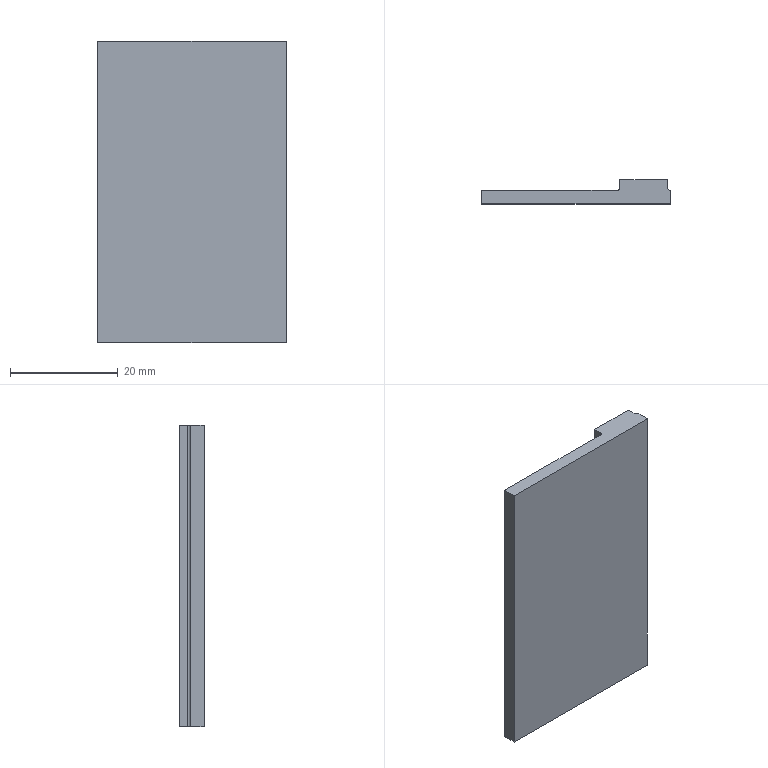Part | NX | features BREP 2 | 2 solids | 22 faces | box 35 x 4.497 x 56 mm | volume 11777 mm3 | plane 18 | cylinder 4 | commonest cylinder face diameters 1 x4
STEP:
#1=CARTESIAN_POINT('',(8.123,0.7486,-4.));
#2=VERTEX_POINT('',#1);
#3=CARTESIAN_POINT('',(8.123,0.7486,52.));
#4=VERTEX_POINT('',#3);
#5=CARTESIAN_POINT('',(8.123,0.7486,0.));
#6=DIRECTION('',(0.,0.,1.));
#7=VECTOR('',#6,1000.);
#8=LINE('',#5,#7);
#9=EDGE_CURVE('',#2,#4,#8,.T.);
#10=ORIENTED_EDGE('',*,*,#9,.T.);
#11=CARTESIAN_POINT('',(8.123,2.249,52.));
#12=VERTEX_POINT('',#11);
#13=CARTESIAN_POINT('',(8.123,28.75,52.));
#14=DIRECTION('',(0.,-1.,0.));
#15=VECTOR('',#14,1000.);
#16=LINE('',#13,#15);
#17=EDGE_CURVE('',#12,#4,#16,.T.);
#18=ORIENTED_EDGE('',*,*,#17,.F.);
#19=CARTESIAN_POINT('',(8.123,2.249,-4.));
#20=VERTEX_POINT('',#19);
#21=CARTESIAN_POINT('',(8.123,2.249,0.));
#22=DIRECTION('',(0.,0.,1.));
#23=VECTOR('',#22,1000.);
#24=LINE('',#21,#23);
#25=EDGE_CURVE('',#20,#12,#24,.T.);
#26=ORIENTED_EDGE('',*,*,#25,.F.);
#27=CARTESIAN_POINT('',(8.123,28.75,-4.));
#28=DIRECTION('',(0.,-1.,0.));
#29=VECTOR('',#28,1000.);
#30=LINE('',#27,#29);
#31=EDGE_CURVE('',#20,#2,#30,.T.);
#32=ORIENTED_EDGE('',*,*,#31,.T.);
#33=EDGE_LOOP('',(#10,#18,#26,#32));
#34=FACE_BOUND('',#33,.T.);
#35=CARTESIAN_POINT('',(8.123,0.7486,0.));
#36=DIRECTION('',(1.,0.,0.));
#37=DIRECTION('',(0.,-1.,0.));
#38=AXIS2_PLACEMENT_3D('',#35,#36,#37);
#39=PLANE('',#38);
#40=ADVANCED_FACE('',(#34),#39,.F.);
#41=ORIENTED_EDGE('',*,*,#25,.T.);
#42=CARTESIAN_POINT('',(17.,2.249,52.));
#43=VERTEX_POINT('',#42);
#44=CARTESIAN_POINT('',(26.573,2.249,52.));
#45=DIRECTION('',(-1.,0.,0.));
#46=VECTOR('',#45,1000.);
#47=LINE('',#44,#46);
#48=EDGE_CURVE('',#43,#12,#47,.T.);
#49=ORIENTED_EDGE('',*,*,#48,.F.);
#50=CARTESIAN_POINT('',(17.,2.249,-4.));
#51=VERTEX_POINT('',#50);
#52=CARTESIAN_POINT('',(17.,2.249,0.));
#53=DIRECTION('',(0.,0.,1.));
#54=VECTOR('',#53,1000.);
#55=LINE('',#52,#54);
#56=EDGE_CURVE('',#51,#43,#55,.T.);
#57=ORIENTED_EDGE('',*,*,#56,.F.);
#58=CARTESIAN_POINT('',(26.573,2.249,-4.));
#59=DIRECTION('',(-1.,0.,0.));
#60=VECTOR('',#59,1000.);
#61=LINE('',#58,#60);
#62=EDGE_CURVE('',#51,#20,#61,.T.);
#63=ORIENTED_EDGE('',*,*,#62,.T.);
#64=EDGE_LOOP('',(#41,#49,#57,#63));
#65=FACE_BOUND('',#64,.T.);
#66=CARTESIAN_POINT('',(8.123,2.249,0.));
#67=DIRECTION('',(0.,-1.,0.));
#68=DIRECTION('',(-1.,0.,0.));
#69=AXIS2_PLACEMENT_3D('',#66,#67,#68);
#70=PLANE('',#69);
#71=ADVANCED_FACE('',(#65),#70,.F.);
#72=ORIENTED_EDGE('',*,*,#56,.T.);
#73=CARTESIAN_POINT('',(17.,0.7486,52.));
#74=VERTEX_POINT('',#73);
#75=CARTESIAN_POINT('',(17.,28.75,52.));
#76=DIRECTION('',(0.,1.,0.));
#77=VECTOR('',#76,1000.);
#78=LINE('',#75,#77);
#79=EDGE_CURVE('',#74,#43,#78,.T.);
#80=ORIENTED_EDGE('',*,*,#79,.F.);
#81=CARTESIAN_POINT('',(17.,0.7486,-4.));
#82=VERTEX_POINT('',#81);
#83=CARTESIAN_POINT('',(17.,0.7486,0.));
#84=DIRECTION('',(0.,0.,1.));
#85=VECTOR('',#84,1000.);
#86=LINE('',#83,#85);
#87=EDGE_CURVE('',#82,#74,#86,.T.);
#88=ORIENTED_EDGE('',*,*,#87,.F.);
#89=CARTESIAN_POINT('',(17.,28.75,-4.));
#90=DIRECTION('',(0.,1.,0.));
#91=VECTOR('',#90,1000.);
#92=LINE('',#89,#91);
#93=EDGE_CURVE('',#82,#51,#92,.T.);
#94=ORIENTED_EDGE('',*,*,#93,.T.);
#95=EDGE_LOOP('',(#72,#80,#88,#94));
#96=FACE_BOUND('',#95,.T.);
#97=CARTESIAN_POINT('',(17.,18.272,0.));
#98=DIRECTION('',(-1.,0.,0.));
#99=DIRECTION('',(0.,1.,0.));
#100=AXIS2_PLACEMENT_3D('',#97,#98,#99);
#101=PLANE('',#100);
#102=ADVANCED_FACE('',(#96),#101,.F.);
#103=ORIENTED_EDGE('',*,*,#87,.T.);
#104=CARTESIAN_POINT('',(17.5,0.2486,52.));
#105=VERTEX_POINT('',#104);
#106=CARTESIAN_POINT('',(17.5,0.7486,52.));
#107=DIRECTION('',(0.,0.,-1.));
#108=DIRECTION('',(1.,0.,0.));
#109=AXIS2_PLACEMENT_3D('',#106,#107,#108);
#110=CIRCLE('',#109,0.5);
#111=EDGE_CURVE('',#105,#74,#110,.T.);
#112=ORIENTED_EDGE('',*,*,#111,.F.);
#113=CARTESIAN_POINT('',(17.5,0.2486,-4.));
#114=VERTEX_POINT('',#113);
#115=CARTESIAN_POINT('',(17.5,0.2486,0.));
#116=DIRECTION('',(0.,0.,1.));
#117=VECTOR('',#116,1000.);
#118=LINE('',#115,#117);
#119=EDGE_CURVE('',#114,#105,#118,.T.);
#120=ORIENTED_EDGE('',*,*,#119,.F.);
#121=CARTESIAN_POINT('',(17.5,0.7486,-4.));
#122=DIRECTION('',(0.,0.,-1.));
#123=DIRECTION('',(1.,0.,0.));
#124=AXIS2_PLACEMENT_3D('',#121,#122,#123);
#125=CIRCLE('',#124,0.5);
#126=EDGE_CURVE('',#114,#82,#125,.T.);
#127=ORIENTED_EDGE('',*,*,#126,.T.);
#128=EDGE_LOOP('',(#103,#112,#120,#127));
#129=FACE_BOUND('',#128,.T.);
#130=CARTESIAN_POINT('',(17.5,0.7486,0.));
#131=DIRECTION('',(0.,0.,1.));
#132=DIRECTION('',(-1.,0.,0.));
#133=AXIS2_PLACEMENT_3D('',#130,#131,#132);
#134=CYLINDRICAL_SURFACE('',#133,0.5);
#135=ADVANCED_FACE('',(#129),#134,.F.);
#136=ORIENTED_EDGE('',*,*,#119,.T.);
#137=CARTESIAN_POINT('',(17.5,-2.243,52.));
#138=VERTEX_POINT('',#137);
#139=CARTESIAN_POINT('',(17.5,28.75,52.));
#140=DIRECTION('',(0.,1.,0.));
#141=VECTOR('',#140,1000.);
#142=LINE('',#139,#141);
#143=EDGE_CURVE('',#138,#105,#142,.T.);
#144=ORIENTED_EDGE('',*,*,#143,.F.);
#145=CARTESIAN_POINT('',(17.5,-2.243,-4.));
#146=VERTEX_POINT('',#145);
#147=CARTESIAN_POINT('',(17.5,-2.243,0.));
#148=DIRECTION('',(0.,0.,1.));
#149=VECTOR('',#148,1000.);
#150=LINE('',#147,#149);
#151=EDGE_CURVE('',#146,#138,#150,.T.);
#152=ORIENTED_EDGE('',*,*,#151,.F.);
#153=CARTESIAN_POINT('',(17.5,28.75,-4.));
#154=DIRECTION('',(0.,1.,0.));
#155=VECTOR('',#154,1000.);
#156=LINE('',#153,#155);
#157=EDGE_CURVE('',#146,#114,#156,.T.);
#158=ORIENTED_EDGE('',*,*,#157,.T.);
#159=EDGE_LOOP('',(#136,#144,#152,#158));
#160=FACE_BOUND('',#159,.T.);
#161=CARTESIAN_POINT('',(17.5,-2.243,0.));
#162=DIRECTION('',(1.,0.,0.));
#163=DIRECTION('',(0.,-1.,0.));
#164=AXIS2_PLACEMENT_3D('',#161,#162,#163);
#165=PLANE('',#164);
#166=ADVANCED_FACE('',(#160),#165,.T.);
#167=ORIENTED_EDGE('',*,*,#151,.T.);
#168=CARTESIAN_POINT('',(-17.5,-2.249,52.));
#169=VERTEX_POINT('',#168);
#170=CARTESIAN_POINT('',(-17.5,-2.249,52.));
#171=DIRECTION('',(1.,0.0001704,0.));
#172=VECTOR('',#171,1000.);
#173=LINE('',#170,#172);
#174=EDGE_CURVE('',#169,#138,#173,.T.);
#175=ORIENTED_EDGE('',*,*,#174,.F.);
#176=CARTESIAN_POINT('',(-17.5,-2.249,-4.));
#177=VERTEX_POINT('',#176);
#178=CARTESIAN_POINT('',(-17.5,-2.249,0.));
#179=DIRECTION('',(0.,0.,1.));
#180=VECTOR('',#179,1000.);
#181=LINE('',#178,#180);
#182=EDGE_CURVE('',#177,#169,#181,.T.);
#183=ORIENTED_EDGE('',*,*,#182,.F.);
#184=CARTESIAN_POINT('',(-17.5,-2.249,-4.));
#185=DIRECTION('',(1.,0.0001704,0.));
#186=VECTOR('',#185,1000.);
#187=LINE('',#184,#186);
#188=EDGE_CURVE('',#177,#146,#187,.T.);
#189=ORIENTED_EDGE('',*,*,#188,.T.);
#190=EDGE_LOOP('',(#167,#175,#183,#189));
#191=FACE_BOUND('',#190,.T.);
#192=CARTESIAN_POINT('',(-17.5,-2.249,0.));
#193=DIRECTION('',(0.0001704,-1.,0.));
#194=DIRECTION('',(-1.,-0.0001704,0.));
#195=AXIS2_PLACEMENT_3D('',#192,#193,#194);
#196=PLANE('',#195);
#197=ADVANCED_FACE('',(#191),#196,.T.);
#198=ORIENTED_EDGE('',*,*,#182,.T.);
#199=CARTESIAN_POINT('',(-17.5,0.2486,52.));
#200=VERTEX_POINT('',#199);
#201=CARTESIAN_POINT('',(-17.5,28.75,52.));
#202=DIRECTION('',(0.,-1.,0.));
#203=VECTOR('',#202,1000.);
#204=LINE('',#201,#203);
#205=EDGE_CURVE('',#200,#169,#204,.T.);
#206=ORIENTED_EDGE('',*,*,#205,.F.);
#207=CARTESIAN_POINT('',(-17.5,0.2486,-4.));
#208=VERTEX_POINT('',#207);
#209=CARTESIAN_POINT('',(-17.5,0.2486,0.));
#210=DIRECTION('',(0.,0.,1.));
#211=VECTOR('',#210,1000.);
#212=LINE('',#209,#211);
#213=EDGE_CURVE('',#208,#200,#212,.T.);
#214=ORIENTED_EDGE('',*,*,#213,.F.);
#215=CARTESIAN_POINT('',(-17.5,28.75,-4.));
#216=DIRECTION('',(0.,-1.,0.));
#217=VECTOR('',#216,1000.);
#218=LINE('',#215,#217);
#219=EDGE_CURVE('',#208,#177,#218,.T.);
#220=ORIENTED_EDGE('',*,*,#219,.T.);
#221=EDGE_LOOP('',(#198,#206,#214,#220));
#222=FACE_BOUND('',#221,.T.);
#223=CARTESIAN_POINT('',(-17.5,0.2486,0.));
#224=DIRECTION('',(-1.,0.,0.));
#225=DIRECTION('',(0.,1.,0.));
#226=AXIS2_PLACEMENT_3D('',#223,#224,#225);
#227=PLANE('',#226);
#228=ADVANCED_FACE('',(#222),#227,.T.);
#229=CARTESIAN_POINT('',(7.623,0.2486,-4.));
#230=VERTEX_POINT('',#229);
#231=CARTESIAN_POINT('',(7.623,0.2486,52.));
#232=VERTEX_POINT('',#231);
#233=CARTESIAN_POINT('',(7.623,0.2486,0.));
#234=DIRECTION('',(0.,0.,1.));
#235=VECTOR('',#234,1000.);
#236=LINE('',#233,#235);
#237=EDGE_CURVE('',#230,#232,#236,.T.);
#238=ORIENTED_EDGE('',*,*,#237,.F.);
#239=CARTESIAN_POINT('',(26.573,0.2486,-4.));
#240=DIRECTION('',(-1.,0.,0.));
#241=VECTOR('',#240,1000.);
#242=LINE('',#239,#241);
#243=EDGE_CURVE('',#230,#208,#242,.T.);
#244=ORIENTED_EDGE('',*,*,#243,.T.);
#245=ORIENTED_EDGE('',*,*,#213,.T.);
#246=CARTESIAN_POINT('',(26.573,0.2486,52.));
#247=DIRECTION('',(-1.,0.,0.));
#248=VECTOR('',#247,1000.);
#249=LINE('',#246,#248);
#250=EDGE_CURVE('',#232,#200,#249,.T.);
#251=ORIENTED_EDGE('',*,*,#250,.F.);
#252=EDGE_LOOP('',(#238,#244,#245,#251));
#253=FACE_BOUND('',#252,.T.);
#254=CARTESIAN_POINT('',(-7.213,0.2486,0.));
#255=DIRECTION('',(0.,-1.,0.));
#256=DIRECTION('',(-1.,0.,0.));
#257=AXIS2_PLACEMENT_3D('',#254,#255,#256);
#258=PLANE('',#257);
#259=ADVANCED_FACE('',(#253),#258,.F.);
#260=CARTESIAN_POINT('',(7.623,0.7486,-4.));
#261=DIRECTION('',(0.,0.,-1.));
#262=DIRECTION('',(1.,0.,0.));
#263=AXIS2_PLACEMENT_3D('',#260,#261,#262);
#264=CIRCLE('',#263,0.5);
#265=EDGE_CURVE('',#2,#230,#264,.T.);
#266=ORIENTED_EDGE('',*,*,#265,.T.);
#267=ORIENTED_EDGE('',*,*,#237,.T.);
#268=CARTESIAN_POINT('',(7.623,0.7486,52.));
#269=DIRECTION('',(0.,0.,-1.));
#270=DIRECTION('',(1.,0.,0.));
#271=AXIS2_PLACEMENT_3D('',#268,#269,#270);
#272=CIRCLE('',#271,0.5);
#273=EDGE_CURVE('',#4,#232,#272,.T.);
#274=ORIENTED_EDGE('',*,*,#273,.F.);
#275=ORIENTED_EDGE('',*,*,#9,.F.);
#276=EDGE_LOOP('',(#266,#267,#274,#275));
#277=FACE_BOUND('',#276,.T.);
#278=CARTESIAN_POINT('',(7.623,0.7486,0.));
#279=DIRECTION('',(0.,0.,1.));
#280=DIRECTION('',(-1.,0.,0.));
#281=AXIS2_PLACEMENT_3D('',#278,#279,#280);
#282=CYLINDRICAL_SURFACE('',#281,0.5);
#283=ADVANCED_FACE('',(#277),#282,.F.);
#284=ORIENTED_EDGE('',*,*,#250,.T.);
#285=ORIENTED_EDGE('',*,*,#205,.T.);
#286=ORIENTED_EDGE('',*,*,#174,.T.);
#287=ORIENTED_EDGE('',*,*,#143,.T.);
#288=ORIENTED_EDGE('',*,*,#111,.T.);
#289=ORIENTED_EDGE('',*,*,#79,.T.);
#290=ORIENTED_EDGE('',*,*,#48,.T.);
#291=ORIENTED_EDGE('',*,*,#17,.T.);
#292=ORIENTED_EDGE('',*,*,#273,.T.);
#293=EDGE_LOOP('',(#284,#285,#286,#287,#288,#289,#290,#291,#292));
#294=FACE_BOUND('',#293,.T.);
#295=CARTESIAN_POINT('',(26.573,28.75,52.));
#296=DIRECTION('',(0.,0.,1.));
#297=DIRECTION('',(-1.,0.,0.));
#298=AXIS2_PLACEMENT_3D('',#295,#296,#297);
#299=PLANE('',#298);
#300=ADVANCED_FACE('',(#294),#299,.T.);
#301=ORIENTED_EDGE('',*,*,#243,.F.);
#302=ORIENTED_EDGE('',*,*,#265,.F.);
#303=ORIENTED_EDGE('',*,*,#31,.F.);
#304=ORIENTED_EDGE('',*,*,#62,.F.);
#305=ORIENTED_EDGE('',*,*,#93,.F.);
#306=ORIENTED_EDGE('',*,*,#126,.F.);
#307=ORIENTED_EDGE('',*,*,#157,.F.);
#308=ORIENTED_EDGE('',*,*,#188,.F.);
#309=ORIENTED_EDGE('',*,*,#219,.F.);
#310=EDGE_LOOP('',(#301,#302,#303,#304,#305,#306,#307,#308,#309));
#311=FACE_BOUND('',#310,.T.);
#312=CARTESIAN_POINT('',(26.573,28.75,-4.));
#313=DIRECTION('',(0.,0.,1.));
#314=DIRECTION('',(-1.,0.,0.));
#315=AXIS2_PLACEMENT_3D('',#312,#313,#314);
#316=PLANE('',#315);
#317=ADVANCED_FACE('',(#311),#316,.F.);
#318=CLOSED_SHELL('',(#40,#71,#102,#135,#166,#197,#228,#259,#283,#300,#317));
#319=MANIFOLD_SOLID_BREP('',#318);
#320=CARTESIAN_POINT('',(8.123,0.7486,-4.));
#321=VERTEX_POINT('',#320);
#322=CARTESIAN_POINT('',(8.123,0.7486,52.));
#323=VERTEX_POINT('',#322);
#324=CARTESIAN_POINT('',(8.123,0.7486,0.));
#325=DIRECTION('',(0.,0.,1.));
#326=VECTOR('',#325,1000.);
#327=LINE('',#324,#326);
#328=EDGE_CURVE('',#321,#323,#327,.T.);
#329=ORIENTED_EDGE('',*,*,#328,.T.);
#330=CARTESIAN_POINT('',(8.123,2.249,52.));
#331=VERTEX_POINT('',#330);
#332=CARTESIAN_POINT('',(8.123,28.75,52.));
#333=DIRECTION('',(0.,-1.,0.));
#334=VECTOR('',#333,1000.);
#335=LINE('',#332,#334);
#336=EDGE_CURVE('',#331,#323,#335,.T.);
#337=ORIENTED_EDGE('',*,*,#336,.F.);
#338=CARTESIAN_POINT('',(8.123,2.249,-4.));
#339=VERTEX_POINT('',#338);
#340=CARTESIAN_POINT('',(8.123,2.249,0.));
#341=DIRECTION('',(0.,0.,1.));
#342=VECTOR('',#341,1000.);
#343=LINE('',#340,#342);
#344=EDGE_CURVE('',#339,#331,#343,.T.);
#345=ORIENTED_EDGE('',*,*,#344,.F.);
#346=CARTESIAN_POINT('',(8.123,28.75,-4.));
#347=DIRECTION('',(0.,-1.,0.));
#348=VECTOR('',#347,1000.);
#349=LINE('',#346,#348);
#350=EDGE_CURVE('',#339,#321,#349,.T.);
#351=ORIENTED_EDGE('',*,*,#350,.T.);
#352=EDGE_LOOP('',(#329,#337,#345,#351));
#353=FACE_BOUND('',#352,.T.);
#354=CARTESIAN_POINT('',(8.123,0.7486,0.));
#355=DIRECTION('',(1.,0.,0.));
#356=DIRECTION('',(0.,-1.,0.));
#357=AXIS2_PLACEMENT_3D('',#354,#355,#356);
#358=PLANE('',#357);
#359=ADVANCED_FACE('',(#353),#358,.F.);
#360=ORIENTED_EDGE('',*,*,#344,.T.);
#361=CARTESIAN_POINT('',(17.,2.249,52.));
#362=VERTEX_POINT('',#361);
#363=CARTESIAN_POINT('',(26.573,2.249,52.));
#364=DIRECTION('',(-1.,0.,0.));
#365=VECTOR('',#364,1000.);
#366=LINE('',#363,#365);
#367=EDGE_CURVE('',#362,#331,#366,.T.);
#368=ORIENTED_EDGE('',*,*,#367,.F.);
#369=CARTESIAN_POINT('',(17.,2.249,-4.));
#370=VERTEX_POINT('',#369);
#371=CARTESIAN_POINT('',(17.,2.249,0.));
#372=DIRECTION('',(0.,0.,1.));
#373=VECTOR('',#372,1000.);
#374=LINE('',#371,#373);
#375=EDGE_CURVE('',#370,#362,#374,.T.);
#376=ORIENTED_EDGE('',*,*,#375,.F.);
#377=CARTESIAN_POINT('',(26.573,2.249,-4.));
#378=DIRECTION('',(-1.,0.,0.));
#379=VECTOR('',#378,1000.);
#380=LINE('',#377,#379);
#381=EDGE_CURVE('',#370,#339,#380,.T.);
#382=ORIENTED_EDGE('',*,*,#381,.T.);
#383=EDGE_LOOP('',(#360,#368,#376,#382));
#384=FACE_BOUND('',#383,.T.);
#385=CARTESIAN_POINT('',(8.123,2.249,0.));
#386=DIRECTION('',(0.,-1.,0.));
#387=DIRECTION('',(-1.,0.,0.));
#388=AXIS2_PLACEMENT_3D('',#385,#386,#387);
#389=PLANE('',#388);
#390=ADVANCED_FACE('',(#384),#389,.F.);
#391=ORIENTED_EDGE('',*,*,#375,.T.);
#392=CARTESIAN_POINT('',(17.,0.7486,52.));
#393=VERTEX_POINT('',#392);
#394=CARTESIAN_POINT('',(17.,28.75,52.));
#395=DIRECTION('',(0.,1.,0.));
#396=VECTOR('',#395,1000.);
#397=LINE('',#394,#396);
#398=EDGE_CURVE('',#393,#362,#397,.T.);
#399=ORIENTED_EDGE('',*,*,#398,.F.);
#400=CARTESIAN_POINT('',(17.,0.7486,-4.));
#401=VERTEX_POINT('',#400);
#402=CARTESIAN_POINT('',(17.,0.7486,0.));
#403=DIRECTION('',(0.,0.,1.));
#404=VECTOR('',#403,1000.);
#405=LINE('',#402,#404);
#406=EDGE_CURVE('',#401,#393,#405,.T.);
#407=ORIENTED_EDGE('',*,*,#406,.F.);
#408=CARTESIAN_POINT('',(17.,28.75,-4.));
#409=DIRECTION('',(0.,1.,0.));
#410=VECTOR('',#409,1000.);
#411=LINE('',#408,#410);
#412=EDGE_CURVE('',#401,#370,#411,.T.);
#413=ORIENTED_EDGE('',*,*,#412,.T.);
#414=EDGE_LOOP('',(#391,#399,#407,#413));
#415=FACE_BOUND('',#414,.T.);
#416=CARTESIAN_POINT('',(17.,18.272,0.));
#417=DIRECTION('',(-1.,0.,0.));
#418=DIRECTION('',(0.,1.,0.));
#419=AXIS2_PLACEMENT_3D('',#416,#417,#418);
#420=PLANE('',#419);
#421=ADVANCED_FACE('',(#415),#420,.F.);
#422=ORIENTED_EDGE('',*,*,#406,.T.);
#423=CARTESIAN_POINT('',(17.5,0.2486,52.));
#424=VERTEX_POINT('',#423);
#425=CARTESIAN_POINT('',(17.5,0.7486,52.));
#426=DIRECTION('',(0.,0.,-1.));
#427=DIRECTION('',(1.,0.,0.));
#428=AXIS2_PLACEMENT_3D('',#425,#426,#427);
#429=CIRCLE('',#428,0.5);
#430=EDGE_CURVE('',#424,#393,#429,.T.);
#431=ORIENTED_EDGE('',*,*,#430,.F.);
#432=CARTESIAN_POINT('',(17.5,0.2486,-4.));
#433=VERTEX_POINT('',#432);
#434=CARTESIAN_POINT('',(17.5,0.2486,0.));
#435=DIRECTION('',(0.,0.,1.));
#436=VECTOR('',#435,1000.);
#437=LINE('',#434,#436);
#438=EDGE_CURVE('',#433,#424,#437,.T.);
#439=ORIENTED_EDGE('',*,*,#438,.F.);
#440=CARTESIAN_POINT('',(17.5,0.7486,-4.));
#441=DIRECTION('',(0.,0.,-1.));
#442=DIRECTION('',(1.,0.,0.));
#443=AXIS2_PLACEMENT_3D('',#440,#441,#442);
#444=CIRCLE('',#443,0.5);
#445=EDGE_CURVE('',#433,#401,#444,.T.);
#446=ORIENTED_EDGE('',*,*,#445,.T.);
#447=EDGE_LOOP('',(#422,#431,#439,#446));
#448=FACE_BOUND('',#447,.T.);
#449=CARTESIAN_POINT('',(17.5,0.7486,0.));
#450=DIRECTION('',(0.,0.,1.));
#451=DIRECTION('',(-1.,0.,0.));
#452=AXIS2_PLACEMENT_3D('',#449,#450,#451);
#453=CYLINDRICAL_SURFACE('',#452,0.5);
#454=ADVANCED_FACE('',(#448),#453,.F.);
#455=ORIENTED_EDGE('',*,*,#438,.T.);
#456=CARTESIAN_POINT('',(17.5,-2.243,52.));
#457=VERTEX_POINT('',#456);
#458=CARTESIAN_POINT('',(17.5,28.75,52.));
#459=DIRECTION('',(0.,1.,0.));
#460=VECTOR('',#459,1000.);
#461=LINE('',#458,#460);
#462=EDGE_CURVE('',#457,#424,#461,.T.);
#463=ORIENTED_EDGE('',*,*,#462,.F.);
#464=CARTESIAN_POINT('',(17.5,-2.243,-4.));
#465=VERTEX_POINT('',#464);
#466=CARTESIAN_POINT('',(17.5,-2.243,0.));
#467=DIRECTION('',(0.,0.,1.));
#468=VECTOR('',#467,1000.);
#469=LINE('',#466,#468);
#470=EDGE_CURVE('',#465,#457,#469,.T.);
#471=ORIENTED_EDGE('',*,*,#470,.F.);
#472=CARTESIAN_POINT('',(17.5,28.75,-4.));
#473=DIRECTION('',(0.,1.,0.));
#474=VECTOR('',#473,1000.);
#475=LINE('',#472,#474);
#476=EDGE_CURVE('',#465,#433,#475,.T.);
#477=ORIENTED_EDGE('',*,*,#476,.T.);
#478=EDGE_LOOP('',(#455,#463,#471,#477));
#479=FACE_BOUND('',#478,.T.);
#480=CARTESIAN_POINT('',(17.5,-2.243,0.));
#481=DIRECTION('',(1.,0.,0.));
#482=DIRECTION('',(0.,-1.,0.));
#483=AXIS2_PLACEMENT_3D('',#480,#481,#482);
#484=PLANE('',#483);
#485=ADVANCED_FACE('',(#479),#484,.T.);
#486=ORIENTED_EDGE('',*,*,#470,.T.);
#487=CARTESIAN_POINT('',(-17.5,-2.249,52.));
#488=VERTEX_POINT('',#487);
#489=CARTESIAN_POINT('',(-17.5,-2.249,52.));
#490=DIRECTION('',(1.,0.0001704,0.));
#491=VECTOR('',#490,1000.);
#492=LINE('',#489,#491);
#493=EDGE_CURVE('',#488,#457,#492,.T.);
#494=ORIENTED_EDGE('',*,*,#493,.F.);
#495=CARTESIAN_POINT('',(-17.5,-2.249,-4.));
#496=VERTEX_POINT('',#495);
#497=CARTESIAN_POINT('',(-17.5,-2.249,0.));
#498=DIRECTION('',(0.,0.,1.));
#499=VECTOR('',#498,1000.);
#500=LINE('',#497,#499);
#501=EDGE_CURVE('',#496,#488,#500,.T.);
#502=ORIENTED_EDGE('',*,*,#501,.F.);
#503=CARTESIAN_POINT('',(-17.5,-2.249,-4.));
#504=DIRECTION('',(1.,0.0001704,0.));
#505=VECTOR('',#504,1000.);
#506=LINE('',#503,#505);
#507=EDGE_CURVE('',#496,#465,#506,.T.);
#508=ORIENTED_EDGE('',*,*,#507,.T.);
#509=EDGE_LOOP('',(#486,#494,#502,#508));
#510=FACE_BOUND('',#509,.T.);
#511=CARTESIAN_POINT('',(-17.5,-2.249,0.));
#512=DIRECTION('',(0.0001704,-1.,0.));
#513=DIRECTION('',(-1.,-0.0001704,0.));
#514=AXIS2_PLACEMENT_3D('',#511,#512,#513);
#515=PLANE('',#514);
#516=ADVANCED_FACE('',(#510),#515,.T.);
#517=ORIENTED_EDGE('',*,*,#501,.T.);
#518=CARTESIAN_POINT('',(-17.5,0.2486,52.));
#519=VERTEX_POINT('',#518);
#520=CARTESIAN_POINT('',(-17.5,28.75,52.));
#521=DIRECTION('',(0.,-1.,0.));
#522=VECTOR('',#521,1000.);
#523=LINE('',#520,#522);
#524=EDGE_CURVE('',#519,#488,#523,.T.);
#525=ORIENTED_EDGE('',*,*,#524,.F.);
#526=CARTESIAN_POINT('',(-17.5,0.2486,-4.));
#527=VERTEX_POINT('',#526);
#528=CARTESIAN_POINT('',(-17.5,0.2486,0.));
#529=DIRECTION('',(0.,0.,1.));
#530=VECTOR('',#529,1000.);
#531=LINE('',#528,#530);
#532=EDGE_CURVE('',#527,#519,#531,.T.);
#533=ORIENTED_EDGE('',*,*,#532,.F.);
#534=CARTESIAN_POINT('',(-17.5,28.75,-4.));
#535=DIRECTION('',(0.,-1.,0.));
#536=VECTOR('',#535,1000.);
#537=LINE('',#534,#536);
#538=EDGE_CURVE('',#527,#496,#537,.T.);
#539=ORIENTED_EDGE('',*,*,#538,.T.);
#540=EDGE_LOOP('',(#517,#525,#533,#539));
#541=FACE_BOUND('',#540,.T.);
#542=CARTESIAN_POINT('',(-17.5,0.2486,0.));
#543=DIRECTION('',(-1.,0.,0.));
#544=DIRECTION('',(0.,1.,0.));
#545=AXIS2_PLACEMENT_3D('',#542,#543,#544);
#546=PLANE('',#545);
#547=ADVANCED_FACE('',(#541),#546,.T.);
#548=CARTESIAN_POINT('',(7.623,0.2486,-4.));
#549=VERTEX_POINT('',#548);
#550=CARTESIAN_POINT('',(7.623,0.2486,52.));
#551=VERTEX_POINT('',#550);
#552=CARTESIAN_POINT('',(7.623,0.2486,0.));
#553=DIRECTION('',(0.,0.,1.));
#554=VECTOR('',#553,1000.);
#555=LINE('',#552,#554);
#556=EDGE_CURVE('',#549,#551,#555,.T.);
#557=ORIENTED_EDGE('',*,*,#556,.F.);
#558=CARTESIAN_POINT('',(26.573,0.2486,-4.));
#559=DIRECTION('',(-1.,0.,0.));
#560=VECTOR('',#559,1000.);
#561=LINE('',#558,#560);
#562=EDGE_CURVE('',#549,#527,#561,.T.);
#563=ORIENTED_EDGE('',*,*,#562,.T.);
#564=ORIENTED_EDGE('',*,*,#532,.T.);
#565=CARTESIAN_POINT('',(26.573,0.2486,52.));
#566=DIRECTION('',(-1.,0.,0.));
#567=VECTOR('',#566,1000.);
#568=LINE('',#565,#567);
#569=EDGE_CURVE('',#551,#519,#568,.T.);
#570=ORIENTED_EDGE('',*,*,#569,.F.);
#571=EDGE_LOOP('',(#557,#563,#564,#570));
#572=FACE_BOUND('',#571,.T.);
#573=CARTESIAN_POINT('',(-7.213,0.2486,0.));
#574=DIRECTION('',(0.,-1.,0.));
#575=DIRECTION('',(-1.,0.,0.));
#576=AXIS2_PLACEMENT_3D('',#573,#574,#575);
#577=PLANE('',#576);
#578=ADVANCED_FACE('',(#572),#577,.F.);
#579=CARTESIAN_POINT('',(7.623,0.7486,-4.));
#580=DIRECTION('',(0.,0.,-1.));
#581=DIRECTION('',(1.,0.,0.));
#582=AXIS2_PLACEMENT_3D('',#579,#580,#581);
#583=CIRCLE('',#582,0.5);
#584=EDGE_CURVE('',#321,#549,#583,.T.);
#585=ORIENTED_EDGE('',*,*,#584,.T.);
#586=ORIENTED_EDGE('',*,*,#556,.T.);
#587=CARTESIAN_POINT('',(7.623,0.7486,52.));
#588=DIRECTION('',(0.,0.,-1.));
#589=DIRECTION('',(1.,0.,0.));
#590=AXIS2_PLACEMENT_3D('',#587,#588,#589);
#591=CIRCLE('',#590,0.5);
#592=EDGE_CURVE('',#323,#551,#591,.T.);
#593=ORIENTED_EDGE('',*,*,#592,.F.);
#594=ORIENTED_EDGE('',*,*,#328,.F.);
#595=EDGE_LOOP('',(#585,#586,#593,#594));
#596=FACE_BOUND('',#595,.T.);
#597=CARTESIAN_POINT('',(7.623,0.7486,0.));
#598=DIRECTION('',(0.,0.,1.));
#599=DIRECTION('',(-1.,0.,0.));
#600=AXIS2_PLACEMENT_3D('',#597,#598,#599);
#601=CYLINDRICAL_SURFACE('',#600,0.5);
#602=ADVANCED_FACE('',(#596),#601,.F.);
#603=ORIENTED_EDGE('',*,*,#569,.T.);
#604=ORIENTED_EDGE('',*,*,#524,.T.);
#605=ORIENTED_EDGE('',*,*,#493,.T.);
#606=ORIENTED_EDGE('',*,*,#462,.T.);
#607=ORIENTED_EDGE('',*,*,#430,.T.);
#608=ORIENTED_EDGE('',*,*,#398,.T.);
#609=ORIENTED_EDGE('',*,*,#367,.T.);
#610=ORIENTED_EDGE('',*,*,#336,.T.);
#611=ORIENTED_EDGE('',*,*,#592,.T.);
#612=EDGE_LOOP('',(#603,#604,#605,#606,#607,#608,#609,#610,#611));
#613=FACE_BOUND('',#612,.T.);
#614=CARTESIAN_POINT('',(26.573,28.75,52.));
#615=DIRECTION('',(0.,0.,1.));
#616=DIRECTION('',(-1.,0.,0.));
#617=AXIS2_PLACEMENT_3D('',#614,#615,#616);
#618=PLANE('',#617);
#619=ADVANCED_FACE('',(#613),#618,.T.);
#620=ORIENTED_EDGE('',*,*,#562,.F.);
#621=ORIENTED_EDGE('',*,*,#584,.F.);
#622=ORIENTED_EDGE('',*,*,#350,.F.);
#623=ORIENTED_EDGE('',*,*,#381,.F.);
#624=ORIENTED_EDGE('',*,*,#412,.F.);
#625=ORIENTED_EDGE('',*,*,#445,.F.);
#626=ORIENTED_EDGE('',*,*,#476,.F.);
#627=ORIENTED_EDGE('',*,*,#507,.F.);
#628=ORIENTED_EDGE('',*,*,#538,.F.);
#629=EDGE_LOOP('',(#620,#621,#622,#623,#624,#625,#626,#627,#628));
#630=FACE_BOUND('',#629,.T.);
#631=CARTESIAN_POINT('',(26.573,28.75,-4.));
#632=DIRECTION('',(0.,0.,1.));
#633=DIRECTION('',(-1.,0.,0.));
#634=AXIS2_PLACEMENT_3D('',#631,#632,#633);
#635=PLANE('',#634);
#636=ADVANCED_FACE('',(#630),#635,.F.);
#637=CLOSED_SHELL('',(#359,#390,#421,#454,#485,#516,#547,#578,#602,#619,#636));
#638=MANIFOLD_SOLID_BREP('',#637);
#639=(LENGTH_UNIT()NAMED_UNIT(*)SI_UNIT(.MILLI.,.METRE.));
#640=UNCERTAINTY_MEASURE_WITH_UNIT(LENGTH_MEASURE(0.00001),#639,'','');
#641=(NAMED_UNIT(*)PLANE_ANGLE_UNIT()SI_UNIT($,.RADIAN.));
#642=(NAMED_UNIT(*)SI_UNIT($,.STERADIAN.)SOLID_ANGLE_UNIT());
#643=(GEOMETRIC_REPRESENTATION_CONTEXT(3)GLOBAL_UNCERTAINTY_ASSIGNED_CONTEXT((#640))GLOBAL_UNIT_ASSIGNED_CONTEXT((#639,#641,#642))REPRESENTATION_CONTEXT('',''));
#644=ADVANCED_BREP_SHAPE_REPRESENTATION('',(#319,#638),#643);